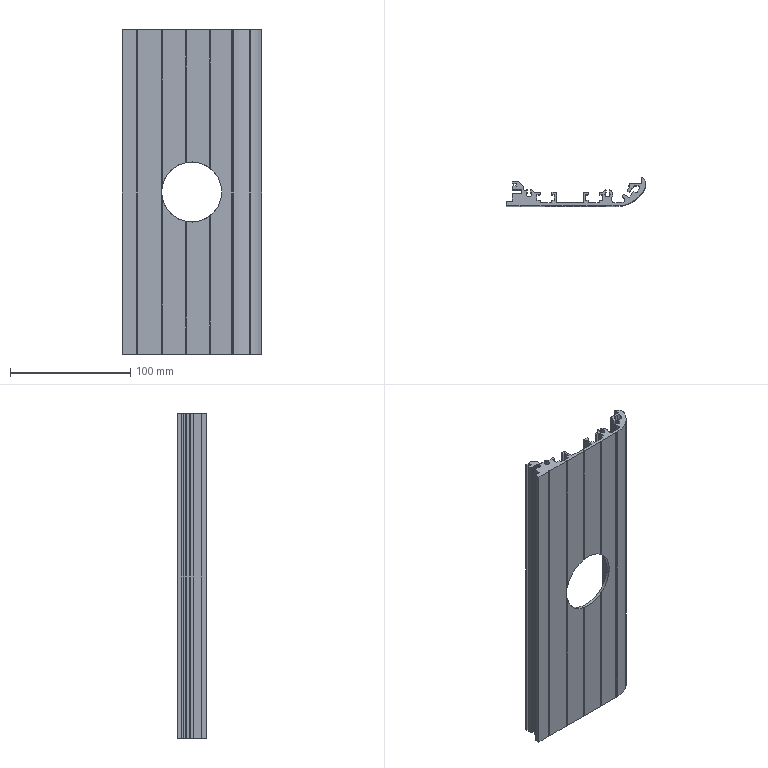Part | SolidWorks | features BaseBody 1 | 1 solid | 232 faces | box 116.267 x 23.727 x 270 mm | volume 194333 mm3 | plane 156 | cylinder 76 | commonest cylinder face diameters 1 x44 4.2 x9 8.7 x5 2 x4 2.4 x2 3 x2